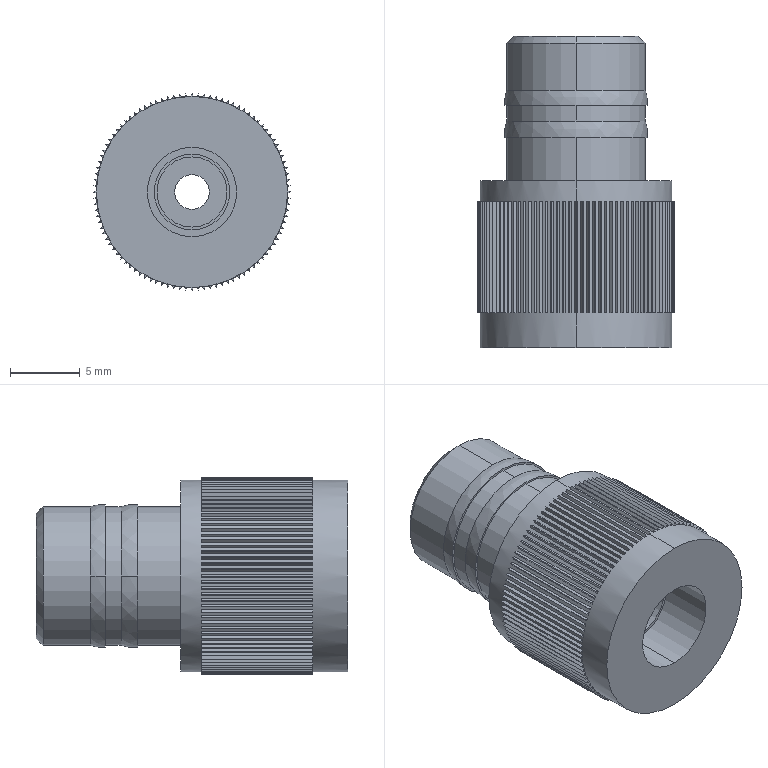Part | SolidWorks | features Chamfer 1, CirPattern 1, ICE 1, Revolution 1 | 1 solid | 430 faces | box 14.16 x 22.4 x 14.16 mm | volume 2205 mm3 | plane 408 | cylinder 16 | spline 4 | cone 2 | commonest cylinder face diameters 10 x6 2.5 x2 5.05 x2 5.45 x2 6.45 x2 13.76 x2